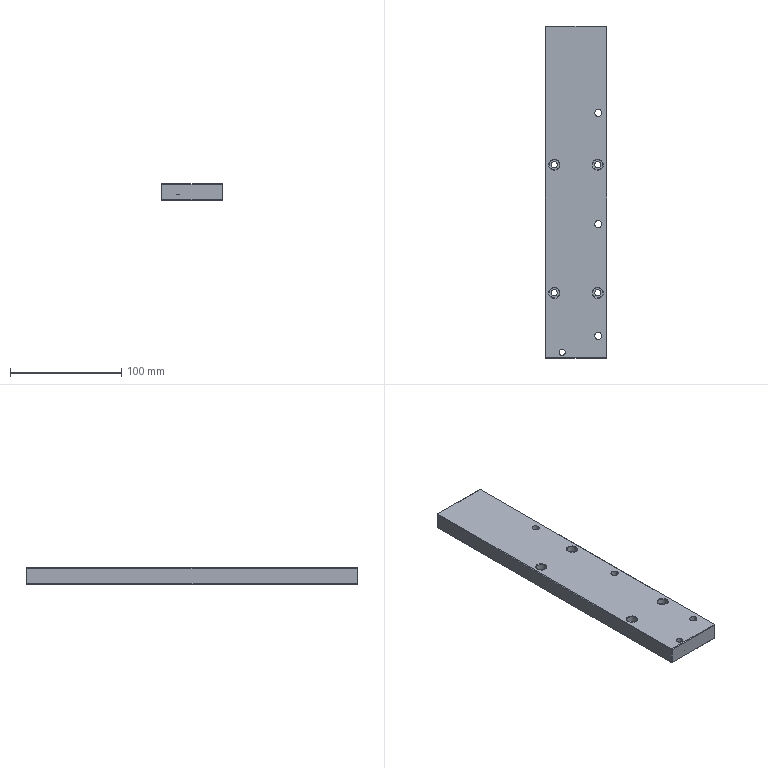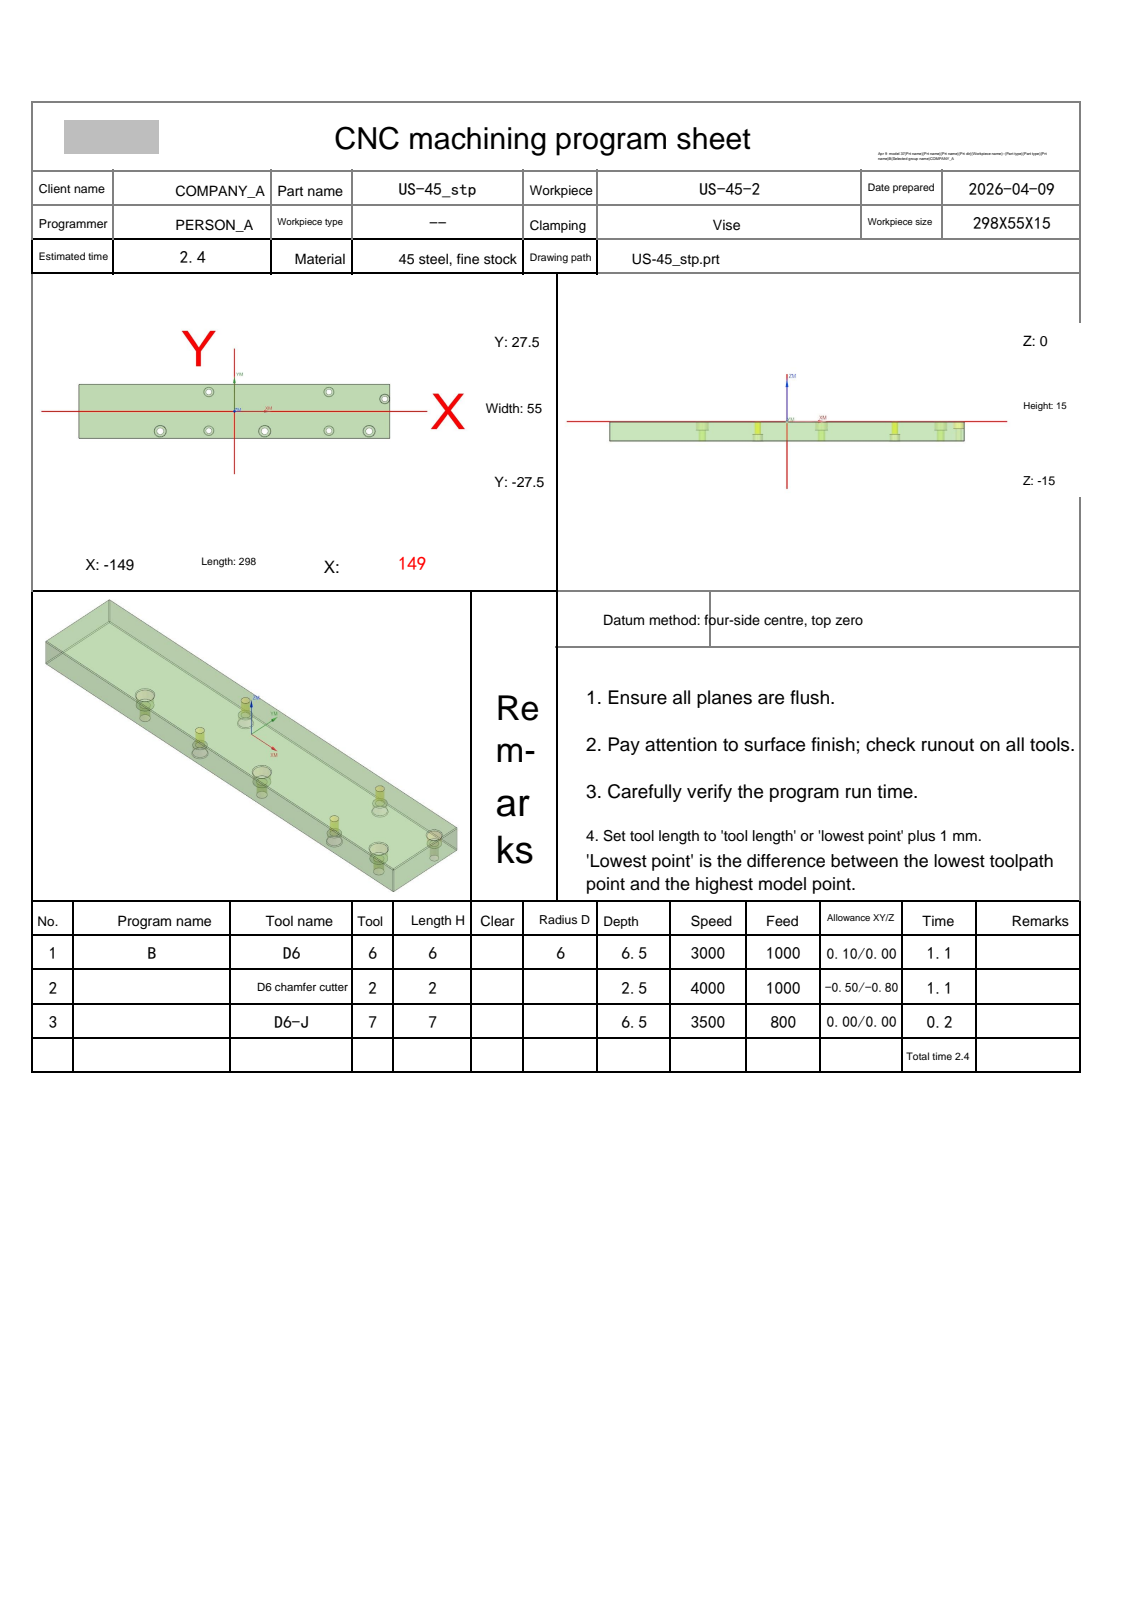NC program | NX | posted by the shop | part box 55 x 298 x 15 mm
Whole program:
%
O0001
(Machine time: 2.92 MIN)
(===Total Tool:3===)
(T6=D6      D=6.   R=0.   D6  H06 Z=-6.5  )
(T2=D6 chamfer cutter   D=6.   R=0.   D-  H02 Z=-2.5  )
(T7=D6-J    D=6.   R=0.   D-  H07 Z=-6.5  )
G80 G90 G17 G49 G40
G91 G28 Z0
M01
N1 T06 M06
(D6  D=6. R=0. H=06 ce=0.10 di=0.00)
G00 G90 G54 X144. Y12.5 M03 S3000
G43 H06 Z20.
M08
Z.8
G41 D06
G01 X143.9 Y12.503 F1000.
G03 X143.295 Y11.805 I.1 J-.698
X144. Y11.1 I.705 J0.0
X144. Y11.1 Z.6 I0.0 J1.4
X144. Y11.1 Z.4 I0.0 J1.4
X144. Y11.1 Z.2 I0.0 J1.4
X144. Y11.1 Z0.0 I0.0 J1.4
X144. Y11.1 Z-.2 I0.0 J1.4
X144. Y11.1 Z-.4 I0.0 J1.4
X144. Y11.1 Z-.6 I0.0 J1.4
X144. Y11.1 Z-.8 I0.0 J1.4
X144. Y11.1 Z-1. I0.0 J1.4
X144. Y11.1 Z-1.2 I0.0 J1.4
X144. Y11.1 Z-1.4 I0.0 J1.4
X144. Y11.1 Z-1.6 I0.0 J1.4
X144. Y11.1 Z-1.8 I0.0 J1.4
X144. Y11.1 Z-2. I0.0 J1.4
X144. Y11.1 Z-2.2 I0.0 J1.4
X144. Y11.1 Z-2.4 I0.0 J1.4
X144. Y11.1 Z-2.6 I0.0 J1.4
X144. Y11.1 Z-2.8 I0.0 J1.4
X144. Y11.1 Z-3. I0.0 J1.4
X144. Y11.1 Z-3.2 I0.0 J1.4
X144. Y11.1 Z-3.4 I0.0 J1.4
X144. Y11.1 Z-3.6 I0.0 J1.4
X144. Y11.1 Z-3.8 I0.0 J1.4
X144. Y11.1 Z-4. I0.0 J1.4
X144. Y11.1 Z-4.2 I0.0 J1.4
X144. Y11.1 Z-4.4 I0.0 J1.4
X144. Y11.1 Z-4.6 I0.0 J1.4
X144. Y11.1 Z-4.8 I0.0 J1.4
X144. Y11.1 Z-5. I0.0 J1.4
X144. Y11.1 Z-5.2 I0.0 J1.4
X144. Y11.1 Z-5.4 I0.0 J1.4
X144.001 Y13.9 Z-5.5 I0.0 J1.4
X142.6 Y12.5 I0.0 J-1.4
X144. Y11.1 I1.4 J0.0
X145.4 Y12.5 I0.0 J1.4
X144.001 Y13.9 I-1.4 J0.0
X143.295 Y13.195 I0.0 J-.705
X143.9 Y12.497 I.705 J0.0
G01 G40 X144. Y12.5
G00 Z20.
G00 G90 X29. Y-20. M03 S3000
Z20.
Z.8
G03 X27.8 Y-21.2 I0.0 J-1.2 F1000.
X29. Y-22.4 I1.2 J0.0
X29. Y-22.4 Z.3 I0.0 J2.4
X29. Y-22.4 Z-.2 I0.0 J2.4
X29. Y-22.4 Z-.7 I0.0 J2.4
X29. Y-22.4 Z-1.2 I0.0 J2.4
X29. Y-22.4 Z-1.7 I0.0 J2.4
X29. Y-22.4 Z-2.2 I0.0 J2.4
X29. Y-22.4 Z-2.7 I0.0 J2.4
X29. Y-22.4 Z-3.2 I0.0 J2.4
X29. Y-22.4 Z-3.7 I0.0 J2.4
X29. Y-22.4 Z-4.2 I0.0 J2.4
X29. Y-22.4 Z-4.7 I0.0 J2.4
X29. Y-22.4 Z-5.2 I0.0 J2.4
X29. Y-22.4 Z-5.7 I0.0 J2.4
X29. Y-22.4 Z-6.2 I0.0 J2.4
X27.59 Y-18.058 Z-6.5 I0.0 J2.4
X26.6 Y-20. I1.41 J-1.942
X29. Y-22.4 I2.4 J0.0
X31.4 Y-20. I0.0 J2.4
X29. Y-17.6 I-2.4 J0.0
X27.59 Y-18.058 I0.0 J-2.4
X27.095 Y-19.029 I.705 J-.971
X28.295 Y-20.229 I1.2 J0.0
X29. Y-20. I0.0 J1.2
G00 Z20.
X-71.
Z.8
G03 X-72.2 Y-21.2 I0.0 J-1.2
X-71. Y-22.4 I1.2 J0.0
X-71. Y-22.4 Z.3 I0.0 J2.4
X-71. Y-22.4 Z-.2 I0.0 J2.4
X-71. Y-22.4 Z-.7 I0.0 J2.4
X-71. Y-22.4 Z-1.2 I0.0 J2.4
X-71. Y-22.4 Z-1.7 I0.0 J2.4
X-71. Y-22.4 Z-2.2 I0.0 J2.4
X-71. Y-22.4 Z-2.7 I0.0 J2.4
X-71. Y-22.4 Z-3.2 I0.0 J2.4
X-71. Y-22.4 Z-3.7 I0.0 J2.4
X-71. Y-22.4 Z-4.2 I0.0 J2.4
X-71. Y-22.4 Z-4.7 I0.0 J2.4
X-71. Y-22.4 Z-5.2 I0.0 J2.4
X-71. Y-22.4 Z-5.7 I0.0 J2.4
X-71. Y-22.4 Z-6.2 I0.0 J2.4
X-72.41 Y-18.058 Z-6.5 I0.0 J2.4
X-73.4 Y-20. I1.41 J-1.942
X-71. Y-22.4 I2.4 J0.0
X-68.6 Y-20. I0.0 J2.4
X-71. Y-17.6 I-2.4 J0.0
X-72.41 Y-18.058 I0.0 J-2.4
X-72.905 Y-19.029 I.705 J-.971
X-71.705 Y-20.229 I1.2 J0.0
X-71. Y-20. I0.0 J1.2
G00 Z20.
X129.
Z.8
G03 X127.8 Y-21.2 I0.0 J-1.2
X129. Y-22.4 I1.2 J0.0
X129. Y-22.4 Z.3 I0.0 J2.4
X129. Y-22.4 Z-.2 I0.0 J2.4
X129. Y-22.4 Z-.7 I0.0 J2.4
X129. Y-22.4 Z-1.2 I0.0 J2.4
X129. Y-22.4 Z-1.7 I0.0 J2.4
X129. Y-22.4 Z-2.2 I0.0 J2.4
X129. Y-22.4 Z-2.7 I0.0 J2.4
X129. Y-22.4 Z-3.2 I0.0 J2.4
X129. Y-22.4 Z-3.7 I0.0 J2.4
X129. Y-22.4 Z-4.2 I0.0 J2.4
X129. Y-22.4 Z-4.7 I0.0 J2.4
X129. Y-22.4 Z-5.2 I0.0 J2.4
X129. Y-22.4 Z-5.7 I0.0 J2.4
X129. Y-22.4 Z-6.2 I0.0 J2.4
X127.59 Y-18.058 Z-6.5 I0.0 J2.4
X126.6 Y-20. I1.41 J-1.942
X129. Y-22.4 I2.4 J0.0
X131.4 Y-20. I0.0 J2.4
X129. Y-17.6 I-2.4 J0.0
X127.59 Y-18.058 I0.0 J-2.4
X127.095 Y-19.029 I.705 J-.971
X128.295 Y-20.229 I1.2 J0.0
X129. Y-20. I0.0 J1.2
G00 Z20.
G91 G28 Z0.0
M05
M09
G91 G28 Z0.0
M01
N2 T02 M06
(D6 chamfer cutter  D=6. R=0. H=02 ce=-0.30 di=-0.80)
G00 G90 G54 X90.094 Y-19.695 M03 S4000
G43 H02 Z20.
M08
Z-1.1
G01 Z-1.6 F600.
X90.09 Y-19.878
X90.089 Y-19.918
G03 X90.5 Y-20.95 I1.5 J0.0
X91.95 Y-19.5 I0.0 J1.45
X90.5 Y-18.05 I-1.45 J0.0
X89.05 Y-19.5 I0.0 J-1.45
X90.5 Y-20.95 I1.45 J0.0
X90.911 Y-19.918 I-1.089 J1.032
G01 X90.91 Y-19.878
X90.906 Y-19.695
Z-1.1
G00 Z20.
X90.094 Y19.305
Z-1.1
G01 Z-1.6
X90.09 Y19.122
X90.089 Y19.082
G03 X90.5 Y18.05 I1.5 J0.0
X91.95 Y19.5 I0.0 J1.45
X90.5 Y20.95 I-1.45 J0.0
X89.05 Y19.5 I0.0 J-1.45
X90.5 Y18.05 I1.45 J0.0
X90.911 Y19.082 I-1.089 J1.032
G01 X90.91 Y19.122
X90.906 Y19.305
Z-1.1
G00 Z20.
X-24.906
Z-1.1
G01 Z-1.6
X-24.91 Y19.122
X-24.911 Y19.082
G03 X-24.5 Y18.05 I1.5 J0.0
X-23.05 Y19.5 I0.0 J1.45
X-24.5 Y20.95 I-1.45 J0.0
X-25.95 Y19.5 I0.0 J-1.45
X-24.5 Y18.05 I1.45 J0.0
X-24.089 Y19.082 I-1.089 J1.032
G01 X-24.09 Y19.122
X-24.094 Y19.305
Z-1.1
G00 Z20.
X-24.906 Y-19.695
Z-1.1
G01 Z-1.6
X-24.91 Y-19.878
X-24.911 Y-19.918
G03 X-24.5 Y-20.95 I1.5 J0.0
X-23.05 Y-19.5 I0.0 J1.45
X-24.5 Y-18.05 I-1.45 J0.0
X-25.95 Y-19.5 I0.0 J-1.45
X-24.5 Y-20.95 I1.45 J0.0
X-24.089 Y-19.918 I-1.089 J1.032
G01 X-24.09 Y-19.878
X-24.094 Y-19.695
Z-1.1
G00 Z20.
G00 G90 X142.5 Y12.5 M03 S3000
Z20.
Z-2.
G01 Z-2.5 F600.
Y11.5
G03 X144. Y10. I1.5 J0.0
X146.5 Y12.5 I0.0 J2.5
X144. Y15. I-2.5 J0.0
X141.5 Y12.5 I0.0 J-2.5
X144. Y10. I2.5 J0.0
X145.5 Y11.5 I0.0 J1.5
G01 Y12.5
Z-2.
G00 Z20.
G00 G90 X126.534 Y-20.411 M03 S3000
Z20.
Z-2.
G01 Z-2.5 F600.
X126. Y-20.5
G03 X129. Y-23.5 I3. J0.0
X132.5 Y-20. I0.0 J3.5
X129. Y-16.5 I-3.5 J0.0
X125.5 Y-20. I0.0 J-3.5
X129. Y-23.5 I3.5 J0.0
X132. Y-20.5 I0.0 J3.
G01 X131.466 Y-20.411
Z-2.
G00 Z20.
X26.534
Z-2.
G01 Z-2.5
X26. Y-20.5
G03 X29. Y-23.5 I3. J0.0
X32.5 Y-20. I0.0 J3.5
X29. Y-16.5 I-3.5 J0.0
X25.5 Y-20. I0.0 J-3.5
X29. Y-23.5 I3.5 J0.0
X32. Y-20.5 I0.0 J3.
G01 X31.466 Y-20.411
Z-2.
G00 Z20.
X-73.466
Z-2.
G01 Z-2.5
X-74. Y-20.5
G03 X-71. Y-23.5 I3. J0.0
X-67.5 Y-20. I0.0 J3.5
X-71. Y-16.5 I-3.5 J0.0
X-74.5 Y-20. I0.0 J-3.5
X-71. Y-23.5 I3.5 J0.0
X-68. Y-20.5 I0.0 J3.
G01 X-68.534 Y-20.411
Z-2.
G00 Z20.
G00 G90 X-150.9 Y29.4 M03 S3500
Z20.
Z.3
G01 Z-1.2 F1000.
G03 X-149.7 Y28.2 I1.2 J0.0
G01 X149.7
Y-28.2
X-149.7
Y28.2
X-149.3
G03 X-148.1 Y29.4 I0.0 J1.2
G01 Z.3
G00 Z20.
G91 G28 Z0.0
M05
M09
G91 G28 Z0.0
M01
N3 T07 M06
(D6-J  D=6. R=0. H=07 ce=0.00 di=0.00)
G00 G90 G54 X144. Y12.5 M03 S3500
G43 H07 Z20.
M08
Z-5.5
G01 X143.669 Y11.451 F600.
X143.653 Y11.347
G03 X144. Y11. I.347 J0.0
X145.5 Y12.5 I0.0 J1.5
X144. Y14. I-1.5 J0.0
X142.5 Y12.5 I0.0 J-1.5
X144. Y11. I1.5 J0.0
X144.491 Y11.083 I0.0 J1.5
X144.724 Y11.41 I-.113 J.328
X144.656 Y11.617 I-.347 J0.0
G01 X144. Y12.5
G00 Z20.
G00 G90 X29. Y-20. M03 S3500
Z20.
Z-6.5
G01 X28.638 Y-22.068 F800.
X28.632 Y-22.132
G03 X29. Y-22.5 I.368 J0.0
X31.5 Y-20. I0.0 J2.5
X29. Y-17.5 I-2.5 J0.0
X26.5 Y-20. I0.0 J-2.5
X29. Y-22.5 I2.5 J0.0
X29.497 Y-22.45 I0.0 J2.5
X29.792 Y-22.09 I-.073 J.361
G01 X29.766 Y-21.955
X29. Y-20.
G00 Z20.
X-71.
Z-6.5
G01 X-71.362 Y-22.068
X-71.368 Y-22.132
G03 X-71. Y-22.5 I.368 J0.0
X-68.5 Y-20. I0.0 J2.5
X-71. Y-17.5 I-2.5 J0.0
X-73.5 Y-20. I0.0 J-2.5
X-71. Y-22.5 I2.5 J0.0
X-70.503 Y-22.45 I0.0 J2.5
X-70.208 Y-22.09 I-.073 J.361
G01 X-70.234 Y-21.955
X-71. Y-20.
G00 Z20.
X129.
Z-6.5
G01 X128.638 Y-22.068
X128.632 Y-22.132
G03 X129. Y-22.5 I.368 J0.0
X131.5 Y-20. I0.0 J2.5
X129. Y-17.5 I-2.5 J0.0
X126.5 Y-20. I0.0 J-2.5
X129. Y-22.5 I2.5 J0.0
X129.497 Y-22.45 I0.0 J2.5
X129.792 Y-22.09 I-.073 J.361
G01 X129.766 Y-21.955
X129. Y-20.
G00 Z20.
M05
M09
G91 G28 Z0.0
G91 G28 Y0.0
M30
%